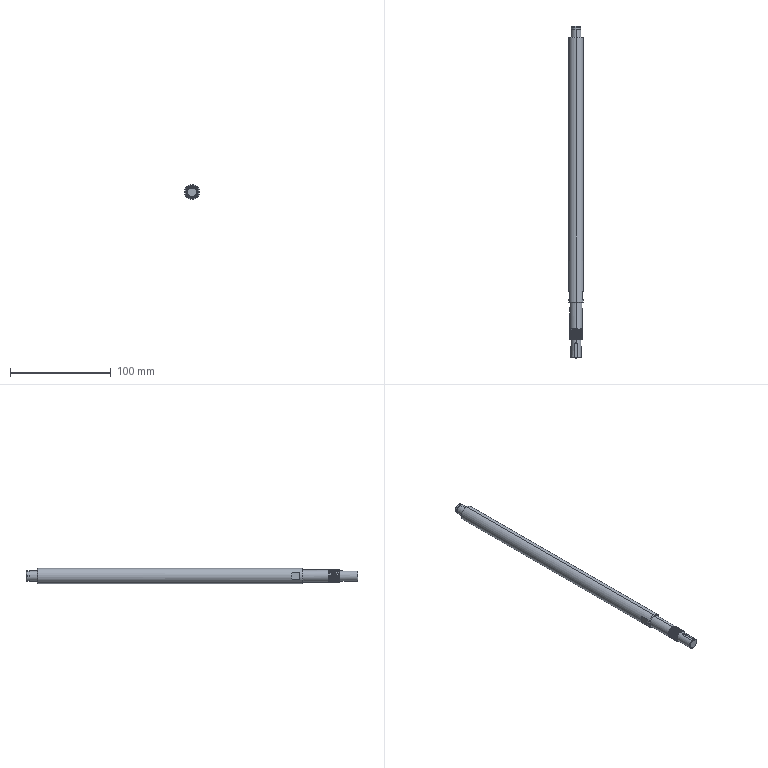Part | STEP file | TBI ball screw 16-20-330 | 1 solid | 112 faces | box 15 x 330 x 15 mm | volume 52902 mm3 | cylinder 83 | plane 19 | cone 7 | spline 3 | commonest cylinder face diameters 12 x71 10 x6 2.9 x2 9.5 x2 15 x2